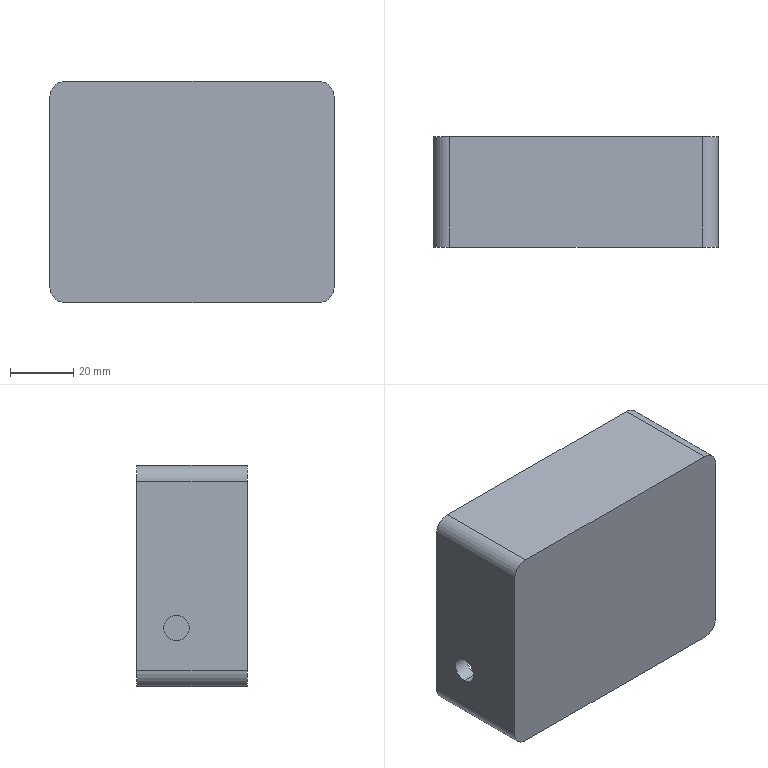Part | SolidWorks | features ICE 2, Extrusion 1, Fillet 1, HoleWzd 1 | 1 solid | 37 faces | box 90 x 35 x 70 mm | volume 61634 mm3 | cylinder 18 | plane 11 | cone 8 | commonest cylinder face diameters 2.5 x8 10 x8 8 x2
STEP:
#1=CARTESIAN_POINT('',(-40.,22.4,-20.5));
#2=VERTEX_POINT('',#1);
#3=CARTESIAN_POINT('',(-40.,22.4,-12.5));
#4=VERTEX_POINT('',#3);
#5=CARTESIAN_POINT('',(-40.,22.4,-16.5));
#6=DIRECTION('',(-1.,0.,0.));
#7=DIRECTION('',(0.,0.,1.));
#8=AXIS2_PLACEMENT_3D('',#5,#6,#7);
#9=CIRCLE('',#8,4.);
#10=EDGE_CURVE('',#2,#4,#9,.T.);
#11=ORIENTED_EDGE('',*,*,#10,.F.);
#12=CARTESIAN_POINT('',(-45.,22.4,-20.5));
#13=VERTEX_POINT('',#12);
#14=CARTESIAN_POINT('',(-35.,22.4,-20.5));
#15=DIRECTION('',(-1.,0.,0.));
#16=VECTOR('',#15,1000.);
#17=LINE('',#14,#16);
#18=EDGE_CURVE('',#2,#13,#17,.T.);
#19=ORIENTED_EDGE('',*,*,#18,.T.);
#20=CARTESIAN_POINT('',(-45.,22.4,-12.5));
#21=VERTEX_POINT('',#20);
#22=CARTESIAN_POINT('',(-45.,22.4,-16.5));
#23=DIRECTION('',(-1.,0.,0.));
#24=DIRECTION('',(0.,0.,1.));
#25=AXIS2_PLACEMENT_3D('',#22,#23,#24);
#26=CIRCLE('',#25,4.);
#27=EDGE_CURVE('',#13,#21,#26,.T.);
#28=ORIENTED_EDGE('',*,*,#27,.T.);
#29=CARTESIAN_POINT('',(-35.,22.4,-12.5));
#30=DIRECTION('',(-1.,0.,0.));
#31=VECTOR('',#30,1000.);
#32=LINE('',#29,#31);
#33=EDGE_CURVE('',#4,#21,#32,.T.);
#34=ORIENTED_EDGE('',*,*,#33,.F.);
#35=EDGE_LOOP('',(#11,#19,#28,#34));
#36=FACE_OUTER_BOUND('',#35,.T.);
#37=CARTESIAN_POINT('',(-35.,22.4,-16.5));
#38=DIRECTION('',(-1.,0.,0.));
#39=DIRECTION('',(0.,0.,1.));
#40=AXIS2_PLACEMENT_3D('',#37,#38,#39);
#41=CYLINDRICAL_SURFACE('',#40,4.);
#42=ADVANCED_FACE('',(#36),#41,.F.);
#43=CARTESIAN_POINT('',(-41.,26.5,-32.25));
#44=VERTEX_POINT('',#43);
#45=CARTESIAN_POINT('',(-41.,26.5,-29.75));
#46=VERTEX_POINT('',#45);
#47=CARTESIAN_POINT('',(-41.,26.5,-31.));
#48=DIRECTION('',(0.,1.,0.));
#49=DIRECTION('',(0.,0.,1.));
#50=AXIS2_PLACEMENT_3D('',#47,#48,#49);
#51=CIRCLE('',#50,1.25);
#52=EDGE_CURVE('',#44,#46,#51,.T.);
#53=ORIENTED_EDGE('',*,*,#52,.F.);
#54=CARTESIAN_POINT('',(-41.,35.,-32.25));
#55=VERTEX_POINT('',#54);
#56=CARTESIAN_POINT('',(-41.,35.,-32.25));
#57=DIRECTION('',(0.,1.,0.));
#58=VECTOR('',#57,1000.);
#59=LINE('',#56,#58);
#60=EDGE_CURVE('',#44,#55,#59,.T.);
#61=ORIENTED_EDGE('',*,*,#60,.T.);
#62=CARTESIAN_POINT('',(-41.,35.,-29.75));
#63=VERTEX_POINT('',#62);
#64=CARTESIAN_POINT('',(-41.,35.,-31.));
#65=DIRECTION('',(0.,1.,0.));
#66=DIRECTION('',(0.,0.,1.));
#67=AXIS2_PLACEMENT_3D('',#64,#65,#66);
#68=CIRCLE('',#67,1.25);
#69=EDGE_CURVE('',#55,#63,#68,.T.);
#70=ORIENTED_EDGE('',*,*,#69,.T.);
#71=CARTESIAN_POINT('',(-41.,35.,-29.75));
#72=DIRECTION('',(0.,1.,0.));
#73=VECTOR('',#72,1000.);
#74=LINE('',#71,#73);
#75=EDGE_CURVE('',#46,#63,#74,.T.);
#76=ORIENTED_EDGE('',*,*,#75,.F.);
#77=EDGE_LOOP('',(#53,#61,#70,#76));
#78=FACE_OUTER_BOUND('',#77,.T.);
#79=CARTESIAN_POINT('',(-41.,35.,-31.));
#80=DIRECTION('',(0.,1.,0.));
#81=DIRECTION('',(0.,0.,1.));
#82=AXIS2_PLACEMENT_3D('',#79,#80,#81);
#83=CYLINDRICAL_SURFACE('',#82,1.25);
#84=ADVANCED_FACE('',(#78),#83,.F.);
#85=CARTESIAN_POINT('',(-41.,25.749,-31.));
#86=VERTEX_POINT('',#85);
#87=CARTESIAN_POINT('',(-41.,26.5,-29.75));
#88=DIRECTION('',(0.,0.515,0.8572));
#89=VECTOR('',#88,1000.);
#90=LINE('',#87,#89);
#91=EDGE_CURVE('',#86,#46,#90,.T.);
#92=ORIENTED_EDGE('',*,*,#91,.F.);
#93=CARTESIAN_POINT('',(-41.,26.5,-32.25));
#94=DIRECTION('',(0.,0.515,-0.8572));
#95=VECTOR('',#94,1000.);
#96=LINE('',#93,#95);
#97=EDGE_CURVE('',#86,#44,#96,.T.);
#98=ORIENTED_EDGE('',*,*,#97,.T.);
#99=ORIENTED_EDGE('',*,*,#52,.T.);
#100=EDGE_LOOP('',(#92,#98,#99));
#101=FACE_OUTER_BOUND('',#100,.T.);
#102=CARTESIAN_POINT('',(-41.,26.5,-31.));
#103=DIRECTION('',(0.,1.,0.));
#104=DIRECTION('',(0.,0.,1.));
#105=AXIS2_PLACEMENT_3D('',#102,#103,#104);
#106=CONICAL_SURFACE('',#105,1.25,1.03);
#107=ADVANCED_FACE('',(#101),#106,.F.);
#108=CARTESIAN_POINT('',(41.,26.5,-32.25));
#109=VERTEX_POINT('',#108);
#110=CARTESIAN_POINT('',(41.,26.5,-29.75));
#111=VERTEX_POINT('',#110);
#112=CARTESIAN_POINT('',(41.,26.5,-31.));
#113=DIRECTION('',(0.,1.,0.));
#114=DIRECTION('',(0.,0.,1.));
#115=AXIS2_PLACEMENT_3D('',#112,#113,#114);
#116=CIRCLE('',#115,1.25);
#117=EDGE_CURVE('',#109,#111,#116,.T.);
#118=ORIENTED_EDGE('',*,*,#117,.F.);
#119=CARTESIAN_POINT('',(41.,35.,-32.25));
#120=VERTEX_POINT('',#119);
#121=CARTESIAN_POINT('',(41.,35.,-32.25));
#122=DIRECTION('',(0.,1.,0.));
#123=VECTOR('',#122,1000.);
#124=LINE('',#121,#123);
#125=EDGE_CURVE('',#109,#120,#124,.T.);
#126=ORIENTED_EDGE('',*,*,#125,.T.);
#127=CARTESIAN_POINT('',(41.,35.,-29.75));
#128=VERTEX_POINT('',#127);
#129=CARTESIAN_POINT('',(41.,35.,-31.));
#130=DIRECTION('',(0.,1.,0.));
#131=DIRECTION('',(0.,0.,1.));
#132=AXIS2_PLACEMENT_3D('',#129,#130,#131);
#133=CIRCLE('',#132,1.25);
#134=EDGE_CURVE('',#120,#128,#133,.T.);
#135=ORIENTED_EDGE('',*,*,#134,.T.);
#136=CARTESIAN_POINT('',(41.,35.,-29.75));
#137=DIRECTION('',(0.,1.,0.));
#138=VECTOR('',#137,1000.);
#139=LINE('',#136,#138);
#140=EDGE_CURVE('',#111,#128,#139,.T.);
#141=ORIENTED_EDGE('',*,*,#140,.F.);
#142=EDGE_LOOP('',(#118,#126,#135,#141));
#143=FACE_OUTER_BOUND('',#142,.T.);
#144=CARTESIAN_POINT('',(41.,35.,-31.));
#145=DIRECTION('',(0.,1.,0.));
#146=DIRECTION('',(0.,0.,1.));
#147=AXIS2_PLACEMENT_3D('',#144,#145,#146);
#148=CYLINDRICAL_SURFACE('',#147,1.25);
#149=ADVANCED_FACE('',(#143),#148,.F.);
#150=CARTESIAN_POINT('',(41.,25.749,-31.));
#151=VERTEX_POINT('',#150);
#152=CARTESIAN_POINT('',(41.,26.5,-29.75));
#153=DIRECTION('',(0.,0.515,0.8572));
#154=VECTOR('',#153,1000.);
#155=LINE('',#152,#154);
#156=EDGE_CURVE('',#151,#111,#155,.T.);
#157=ORIENTED_EDGE('',*,*,#156,.F.);
#158=CARTESIAN_POINT('',(41.,26.5,-32.25));
#159=DIRECTION('',(0.,0.515,-0.8572));
#160=VECTOR('',#159,1000.);
#161=LINE('',#158,#160);
#162=EDGE_CURVE('',#151,#109,#161,.T.);
#163=ORIENTED_EDGE('',*,*,#162,.T.);
#164=ORIENTED_EDGE('',*,*,#117,.T.);
#165=EDGE_LOOP('',(#157,#163,#164));
#166=FACE_OUTER_BOUND('',#165,.T.);
#167=CARTESIAN_POINT('',(41.,26.5,-31.));
#168=DIRECTION('',(0.,1.,0.));
#169=DIRECTION('',(0.,0.,1.));
#170=AXIS2_PLACEMENT_3D('',#167,#168,#169);
#171=CONICAL_SURFACE('',#170,1.25,1.03);
#172=ADVANCED_FACE('',(#166),#171,.F.);
#173=CARTESIAN_POINT('',(41.,26.5,29.75));
#174=VERTEX_POINT('',#173);
#175=CARTESIAN_POINT('',(41.,26.5,32.25));
#176=VERTEX_POINT('',#175);
#177=CARTESIAN_POINT('',(41.,26.5,31.));
#178=DIRECTION('',(0.,1.,0.));
#179=DIRECTION('',(0.,0.,1.));
#180=AXIS2_PLACEMENT_3D('',#177,#178,#179);
#181=CIRCLE('',#180,1.25);
#182=EDGE_CURVE('',#174,#176,#181,.T.);
#183=ORIENTED_EDGE('',*,*,#182,.F.);
#184=CARTESIAN_POINT('',(41.,35.,29.75));
#185=VERTEX_POINT('',#184);
#186=CARTESIAN_POINT('',(41.,35.,29.75));
#187=DIRECTION('',(0.,1.,0.));
#188=VECTOR('',#187,1000.);
#189=LINE('',#186,#188);
#190=EDGE_CURVE('',#174,#185,#189,.T.);
#191=ORIENTED_EDGE('',*,*,#190,.T.);
#192=CARTESIAN_POINT('',(41.,35.,32.25));
#193=VERTEX_POINT('',#192);
#194=CARTESIAN_POINT('',(41.,35.,31.));
#195=DIRECTION('',(0.,1.,0.));
#196=DIRECTION('',(0.,0.,1.));
#197=AXIS2_PLACEMENT_3D('',#194,#195,#196);
#198=CIRCLE('',#197,1.25);
#199=EDGE_CURVE('',#185,#193,#198,.T.);
#200=ORIENTED_EDGE('',*,*,#199,.T.);
#201=CARTESIAN_POINT('',(41.,35.,32.25));
#202=DIRECTION('',(0.,1.,0.));
#203=VECTOR('',#202,1000.);
#204=LINE('',#201,#203);
#205=EDGE_CURVE('',#176,#193,#204,.T.);
#206=ORIENTED_EDGE('',*,*,#205,.F.);
#207=EDGE_LOOP('',(#183,#191,#200,#206));
#208=FACE_OUTER_BOUND('',#207,.T.);
#209=CARTESIAN_POINT('',(41.,35.,31.));
#210=DIRECTION('',(0.,1.,0.));
#211=DIRECTION('',(0.,0.,1.));
#212=AXIS2_PLACEMENT_3D('',#209,#210,#211);
#213=CYLINDRICAL_SURFACE('',#212,1.25);
#214=ADVANCED_FACE('',(#208),#213,.F.);
#215=CARTESIAN_POINT('',(41.,25.749,31.));
#216=VERTEX_POINT('',#215);
#217=CARTESIAN_POINT('',(41.,26.5,32.25));
#218=DIRECTION('',(0.,0.515,0.8572));
#219=VECTOR('',#218,1000.);
#220=LINE('',#217,#219);
#221=EDGE_CURVE('',#216,#176,#220,.T.);
#222=ORIENTED_EDGE('',*,*,#221,.F.);
#223=CARTESIAN_POINT('',(41.,26.5,29.75));
#224=DIRECTION('',(0.,0.515,-0.8572));
#225=VECTOR('',#224,1000.);
#226=LINE('',#223,#225);
#227=EDGE_CURVE('',#216,#174,#226,.T.);
#228=ORIENTED_EDGE('',*,*,#227,.T.);
#229=ORIENTED_EDGE('',*,*,#182,.T.);
#230=EDGE_LOOP('',(#222,#228,#229));
#231=FACE_OUTER_BOUND('',#230,.T.);
#232=CARTESIAN_POINT('',(41.,26.5,31.));
#233=DIRECTION('',(0.,1.,0.));
#234=DIRECTION('',(0.,0.,1.));
#235=AXIS2_PLACEMENT_3D('',#232,#233,#234);
#236=CONICAL_SURFACE('',#235,1.25,1.03);
#237=ADVANCED_FACE('',(#231),#236,.F.);
#238=CARTESIAN_POINT('',(-41.,26.5,29.75));
#239=VERTEX_POINT('',#238);
#240=CARTESIAN_POINT('',(-41.,26.5,32.25));
#241=VERTEX_POINT('',#240);
#242=CARTESIAN_POINT('',(-41.,26.5,31.));
#243=DIRECTION('',(0.,1.,0.));
#244=DIRECTION('',(0.,0.,1.));
#245=AXIS2_PLACEMENT_3D('',#242,#243,#244);
#246=CIRCLE('',#245,1.25);
#247=EDGE_CURVE('',#239,#241,#246,.T.);
#248=ORIENTED_EDGE('',*,*,#247,.F.);
#249=CARTESIAN_POINT('',(-41.,35.,29.75));
#250=VERTEX_POINT('',#249);
#251=CARTESIAN_POINT('',(-41.,35.,29.75));
#252=DIRECTION('',(0.,1.,0.));
#253=VECTOR('',#252,1000.);
#254=LINE('',#251,#253);
#255=EDGE_CURVE('',#239,#250,#254,.T.);
#256=ORIENTED_EDGE('',*,*,#255,.T.);
#257=CARTESIAN_POINT('',(-41.,35.,32.25));
#258=VERTEX_POINT('',#257);
#259=CARTESIAN_POINT('',(-41.,35.,31.));
#260=DIRECTION('',(0.,1.,0.));
#261=DIRECTION('',(0.,0.,1.));
#262=AXIS2_PLACEMENT_3D('',#259,#260,#261);
#263=CIRCLE('',#262,1.25);
#264=EDGE_CURVE('',#250,#258,#263,.T.);
#265=ORIENTED_EDGE('',*,*,#264,.T.);
#266=CARTESIAN_POINT('',(-41.,35.,32.25));
#267=DIRECTION('',(0.,1.,0.));
#268=VECTOR('',#267,1000.);
#269=LINE('',#266,#268);
#270=EDGE_CURVE('',#241,#258,#269,.T.);
#271=ORIENTED_EDGE('',*,*,#270,.F.);
#272=EDGE_LOOP('',(#248,#256,#265,#271));
#273=FACE_OUTER_BOUND('',#272,.T.);
#274=CARTESIAN_POINT('',(-41.,35.,31.));
#275=DIRECTION('',(0.,1.,0.));
#276=DIRECTION('',(0.,0.,1.));
#277=AXIS2_PLACEMENT_3D('',#274,#275,#276);
#278=CYLINDRICAL_SURFACE('',#277,1.25);
#279=ADVANCED_FACE('',(#273),#278,.F.);
#280=CARTESIAN_POINT('',(-41.,25.749,31.));
#281=VERTEX_POINT('',#280);
#282=CARTESIAN_POINT('',(-41.,26.5,32.25));
#283=DIRECTION('',(0.,0.515,0.8572));
#284=VECTOR('',#283,1000.);
#285=LINE('',#282,#284);
#286=EDGE_CURVE('',#281,#241,#285,.T.);
#287=ORIENTED_EDGE('',*,*,#286,.F.);
#288=CARTESIAN_POINT('',(-41.,26.5,29.75));
#289=DIRECTION('',(0.,0.515,-0.8572));
#290=VECTOR('',#289,1000.);
#291=LINE('',#288,#290);
#292=EDGE_CURVE('',#281,#239,#291,.T.);
#293=ORIENTED_EDGE('',*,*,#292,.T.);
#294=ORIENTED_EDGE('',*,*,#247,.T.);
#295=EDGE_LOOP('',(#287,#293,#294));
#296=FACE_OUTER_BOUND('',#295,.T.);
#297=CARTESIAN_POINT('',(-41.,26.5,31.));
#298=DIRECTION('',(0.,1.,0.));
#299=DIRECTION('',(0.,0.,1.));
#300=AXIS2_PLACEMENT_3D('',#297,#298,#299);
#301=CONICAL_SURFACE('',#300,1.25,1.03);
#302=ADVANCED_FACE('',(#296),#301,.F.);
#303=CARTESIAN_POINT('',(-41.,35.,-31.));
#304=DIRECTION('',(0.,1.,0.));
#305=DIRECTION('',(0.,0.,1.));
#306=AXIS2_PLACEMENT_3D('',#303,#304,#305);
#307=CIRCLE('',#306,1.25);
#308=EDGE_CURVE('',#63,#55,#307,.T.);
#309=ORIENTED_EDGE('',*,*,#308,.F.);
#310=ORIENTED_EDGE('',*,*,#69,.F.);
#311=EDGE_LOOP('',(#309,#310));
#312=FACE_BOUND('',#311,.T.);
#313=CARTESIAN_POINT('',(41.,35.,-31.));
#314=DIRECTION('',(0.,1.,0.));
#315=DIRECTION('',(0.,0.,1.));
#316=AXIS2_PLACEMENT_3D('',#313,#314,#315);
#317=CIRCLE('',#316,1.25);
#318=EDGE_CURVE('',#128,#120,#317,.T.);
#319=ORIENTED_EDGE('',*,*,#318,.F.);
#320=ORIENTED_EDGE('',*,*,#134,.F.);
#321=EDGE_LOOP('',(#319,#320));
#322=FACE_BOUND('',#321,.T.);
#323=CARTESIAN_POINT('',(-41.,35.,31.));
#324=DIRECTION('',(0.,1.,0.));
#325=DIRECTION('',(0.,0.,1.));
#326=AXIS2_PLACEMENT_3D('',#323,#324,#325);
#327=CIRCLE('',#326,1.25);
#328=EDGE_CURVE('',#258,#250,#327,.T.);
#329=ORIENTED_EDGE('',*,*,#328,.F.);
#330=ORIENTED_EDGE('',*,*,#264,.F.);
#331=EDGE_LOOP('',(#329,#330));
#332=FACE_BOUND('',#331,.T.);
#333=CARTESIAN_POINT('',(35.,35.,-30.));
#334=VERTEX_POINT('',#333);
#335=CARTESIAN_POINT('',(-35.,35.,-30.));
#336=VERTEX_POINT('',#335);
#337=CARTESIAN_POINT('',(-40.,35.,-30.));
#338=DIRECTION('',(-1.,0.,0.));
#339=VECTOR('',#338,1000.);
#340=LINE('',#337,#339);
#341=EDGE_CURVE('',#334,#336,#340,.T.);
#342=ORIENTED_EDGE('',*,*,#341,.F.);
#343=CARTESIAN_POINT('',(40.,35.,-25.));
#344=VERTEX_POINT('',#343);
#345=CARTESIAN_POINT('',(35.,35.,-25.));
#346=DIRECTION('',(0.,-1.,0.));
#347=DIRECTION('',(0.,0.,-1.));
#348=AXIS2_PLACEMENT_3D('',#345,#346,#347);
#349=CIRCLE('',#348,5.);
#350=EDGE_CURVE('',#334,#344,#349,.T.);
#351=ORIENTED_EDGE('',*,*,#350,.T.);
#352=CARTESIAN_POINT('',(40.,35.,25.));
#353=VERTEX_POINT('',#352);
#354=CARTESIAN_POINT('',(40.,35.,30.));
#355=DIRECTION('',(0.,0.,-1.));
#356=VECTOR('',#355,1000.);
#357=LINE('',#354,#356);
#358=EDGE_CURVE('',#353,#344,#357,.T.);
#359=ORIENTED_EDGE('',*,*,#358,.F.);
#360=CARTESIAN_POINT('',(35.,35.,30.));
#361=VERTEX_POINT('',#360);
#362=CARTESIAN_POINT('',(35.,35.,25.));
#363=DIRECTION('',(0.,-1.,0.));
#364=DIRECTION('',(0.,0.,-1.));
#365=AXIS2_PLACEMENT_3D('',#362,#363,#364);
#366=CIRCLE('',#365,5.);
#367=EDGE_CURVE('',#353,#361,#366,.T.);
#368=ORIENTED_EDGE('',*,*,#367,.T.);
#369=CARTESIAN_POINT('',(-35.,35.,30.));
#370=VERTEX_POINT('',#369);
#371=CARTESIAN_POINT('',(-40.,35.,30.));
#372=DIRECTION('',(1.,0.,0.));
#373=VECTOR('',#372,1000.);
#374=LINE('',#371,#373);
#375=EDGE_CURVE('',#370,#361,#374,.T.);
#376=ORIENTED_EDGE('',*,*,#375,.F.);
#377=CARTESIAN_POINT('',(-40.,35.,25.));
#378=VERTEX_POINT('',#377);
#379=CARTESIAN_POINT('',(-35.,35.,25.));
#380=DIRECTION('',(0.,-1.,0.));
#381=DIRECTION('',(0.,0.,-1.));
#382=AXIS2_PLACEMENT_3D('',#379,#380,#381);
#383=CIRCLE('',#382,5.);
#384=EDGE_CURVE('',#370,#378,#383,.T.);
#385=ORIENTED_EDGE('',*,*,#384,.T.);
#386=CARTESIAN_POINT('',(-40.,35.,-25.));
#387=VERTEX_POINT('',#386);
#388=CARTESIAN_POINT('',(-40.,35.,30.));
#389=DIRECTION('',(0.,0.,1.));
#390=VECTOR('',#389,1000.);
#391=LINE('',#388,#390);
#392=EDGE_CURVE('',#387,#378,#391,.T.);
#393=ORIENTED_EDGE('',*,*,#392,.F.);
#394=CARTESIAN_POINT('',(-35.,35.,-25.));
#395=DIRECTION('',(0.,-1.,0.));
#396=DIRECTION('',(0.,0.,-1.));
#397=AXIS2_PLACEMENT_3D('',#394,#395,#396);
#398=CIRCLE('',#397,5.);
#399=EDGE_CURVE('',#387,#336,#398,.T.);
#400=ORIENTED_EDGE('',*,*,#399,.T.);
#401=EDGE_LOOP('',(#342,#351,#359,#368,#376,#385,#393,#400));
#402=FACE_BOUND('',#401,.T.);
#403=CARTESIAN_POINT('',(45.,35.,30.));
#404=VERTEX_POINT('',#403);
#405=CARTESIAN_POINT('',(45.,35.,-30.));
#406=VERTEX_POINT('',#405);
#407=CARTESIAN_POINT('',(45.,35.,35.));
#408=DIRECTION('',(0.,0.,-1.));
#409=VECTOR('',#408,1000.);
#410=LINE('',#407,#409);
#411=EDGE_CURVE('',#404,#406,#410,.T.);
#412=ORIENTED_EDGE('',*,*,#411,.T.);
#413=CARTESIAN_POINT('',(40.,35.,-35.));
#414=VERTEX_POINT('',#413);
#415=CARTESIAN_POINT('',(40.,35.,-30.));
#416=DIRECTION('',(0.,1.,0.));
#417=DIRECTION('',(0.,0.,-1.));
#418=AXIS2_PLACEMENT_3D('',#415,#416,#417);
#419=CIRCLE('',#418,5.);
#420=EDGE_CURVE('',#406,#414,#419,.T.);
#421=ORIENTED_EDGE('',*,*,#420,.T.);
#422=CARTESIAN_POINT('',(-40.,35.,-35.));
#423=VERTEX_POINT('',#422);
#424=CARTESIAN_POINT('',(-45.,35.,-35.));
#425=DIRECTION('',(-1.,0.,0.));
#426=VECTOR('',#425,1000.);
#427=LINE('',#424,#426);
#428=EDGE_CURVE('',#414,#423,#427,.T.);
#429=ORIENTED_EDGE('',*,*,#428,.T.);
#430=CARTESIAN_POINT('',(-45.,35.,-30.));
#431=VERTEX_POINT('',#430);
#432=CARTESIAN_POINT('',(-40.,35.,-30.));
#433=DIRECTION('',(0.,1.,0.));
#434=DIRECTION('',(0.,0.,-1.));
#435=AXIS2_PLACEMENT_3D('',#432,#433,#434);
#436=CIRCLE('',#435,5.);
#437=EDGE_CURVE('',#423,#431,#436,.T.);
#438=ORIENTED_EDGE('',*,*,#437,.T.);
#439=CARTESIAN_POINT('',(-45.,35.,30.));
#440=VERTEX_POINT('',#439);
#441=CARTESIAN_POINT('',(-45.,35.,35.));
#442=DIRECTION('',(0.,0.,1.));
#443=VECTOR('',#442,1000.);
#444=LINE('',#441,#443);
#445=EDGE_CURVE('',#431,#440,#444,.T.);
#446=ORIENTED_EDGE('',*,*,#445,.T.);
#447=CARTESIAN_POINT('',(-40.,35.,35.));
#448=VERTEX_POINT('',#447);
#449=CARTESIAN_POINT('',(-40.,35.,30.));
#450=DIRECTION('',(0.,1.,0.));
#451=DIRECTION('',(0.,0.,-1.));
#452=AXIS2_PLACEMENT_3D('',#449,#450,#451);
#453=CIRCLE('',#452,5.);
#454=EDGE_CURVE('',#440,#448,#453,.T.);
#455=ORIENTED_EDGE('',*,*,#454,.T.);
#456=CARTESIAN_POINT('',(40.,35.,35.));
#457=VERTEX_POINT('',#456);
#458=CARTESIAN_POINT('',(-45.,35.,35.));
#459=DIRECTION('',(1.,0.,0.));
#460=VECTOR('',#459,1000.);
#461=LINE('',#458,#460);
#462=EDGE_CURVE('',#448,#457,#461,.T.);
#463=ORIENTED_EDGE('',*,*,#462,.T.);
#464=CARTESIAN_POINT('',(40.,35.,30.));
#465=DIRECTION('',(0.,1.,0.));
#466=DIRECTION('',(0.,0.,-1.));
#467=AXIS2_PLACEMENT_3D('',#464,#465,#466);
#468=CIRCLE('',#467,5.);
#469=EDGE_CURVE('',#457,#404,#468,.T.);
#470=ORIENTED_EDGE('',*,*,#469,.T.);
#471=EDGE_LOOP('',(#412,#421,#429,#438,#446,#455,#463,#470));
#472=FACE_OUTER_BOUND('',#471,.T.);
#473=CARTESIAN_POINT('',(41.,35.,31.));
#474=DIRECTION('',(0.,1.,0.));
#475=DIRECTION('',(0.,0.,1.));
#476=AXIS2_PLACEMENT_3D('',#473,#474,#475);
#477=CIRCLE('',#476,1.25);
#478=EDGE_CURVE('',#193,#185,#477,.T.);
#479=ORIENTED_EDGE('',*,*,#478,.F.);
#480=ORIENTED_EDGE('',*,*,#199,.F.);
#481=EDGE_LOOP('',(#479,#480));
#482=FACE_BOUND('',#481,.T.);
#483=CARTESIAN_POINT('',(0.,35.,0.));
#484=DIRECTION('',(0.,-1.,0.));
#485=DIRECTION('',(0.,0.,-1.));
#486=AXIS2_PLACEMENT_3D('',#483,#484,#485);
#487=PLANE('',#486);
#488=ADVANCED_FACE('',(#312,#322,#332,#402,#472,#482),#487,.F.);
#489=CARTESIAN_POINT('',(45.,0.,30.));
#490=VERTEX_POINT('',#489);
#491=CARTESIAN_POINT('',(45.,0.,-30.));
#492=VERTEX_POINT('',#491);
#493=CARTESIAN_POINT('',(45.,0.,35.));
#494=DIRECTION('',(0.,0.,-1.));
#495=VECTOR('',#494,1000.);
#496=LINE('',#493,#495);
#497=EDGE_CURVE('',#490,#492,#496,.T.);
#498=ORIENTED_EDGE('',*,*,#497,.T.);
#499=CARTESIAN_POINT('',(45.,35.,-30.));
#500=DIRECTION('',(0.,1.,0.));
#501=VECTOR('',#500,1000.);
#502=LINE('',#499,#501);
#503=EDGE_CURVE('',#492,#406,#502,.T.);
#504=ORIENTED_EDGE('',*,*,#503,.T.);
#505=ORIENTED_EDGE('',*,*,#411,.F.);
#506=CARTESIAN_POINT('',(45.,35.,30.));
#507=DIRECTION('',(0.,-1.,0.));
#508=VECTOR('',#507,1000.);
#509=LINE('',#506,#508);
#510=EDGE_CURVE('',#404,#490,#509,.T.);
#511=ORIENTED_EDGE('',*,*,#510,.T.);
#512=EDGE_LOOP('',(#498,#504,#505,#511));
#513=FACE_OUTER_BOUND('',#512,.T.);
#514=CARTESIAN_POINT('',(45.,35.,35.));
#515=DIRECTION('',(-1.,0.,0.));
#516=DIRECTION('',(0.,0.,1.));
#517=AXIS2_PLACEMENT_3D('',#514,#515,#516);
#518=PLANE('',#517);
#519=ADVANCED_FACE('',(#513),#518,.F.);
#520=ORIENTED_EDGE('',*,*,#428,.F.);
#521=CARTESIAN_POINT('',(40.,0.,-35.));
#522=VERTEX_POINT('',#521);
#523=CARTESIAN_POINT('',(40.,35.,-35.));
#524=DIRECTION('',(0.,-1.,0.));
#525=VECTOR('',#524,1000.);
#526=LINE('',#523,#525);
#527=EDGE_CURVE('',#414,#522,#526,.T.);
#528=ORIENTED_EDGE('',*,*,#527,.T.);
#529=CARTESIAN_POINT('',(-40.,0.,-35.));
#530=VERTEX_POINT('',#529);
#531=CARTESIAN_POINT('',(-45.,0.,-35.));
#532=DIRECTION('',(-1.,0.,0.));
#533=VECTOR('',#532,1000.);
#534=LINE('',#531,#533);
#535=EDGE_CURVE('',#522,#530,#534,.T.);
#536=ORIENTED_EDGE('',*,*,#535,.T.);
#537=CARTESIAN_POINT('',(-40.,35.,-35.));
#538=DIRECTION('',(0.,1.,0.));
#539=VECTOR('',#538,1000.);
#540=LINE('',#537,#539);
#541=EDGE_CURVE('',#530,#423,#540,.T.);
#542=ORIENTED_EDGE('',*,*,#541,.T.);
#543=EDGE_LOOP('',(#520,#528,#536,#542));
#544=FACE_OUTER_BOUND('',#543,.T.);
#545=CARTESIAN_POINT('',(-45.,35.,-35.));
#546=DIRECTION('',(0.,0.,1.));
#547=DIRECTION('',(1.,0.,0.));
#548=AXIS2_PLACEMENT_3D('',#545,#546,#547);
#549=PLANE('',#548);
#550=ADVANCED_FACE('',(#544),#549,.F.);
#551=CARTESIAN_POINT('',(-45.,22.4,-16.5));
#552=DIRECTION('',(-1.,0.,0.));
#553=DIRECTION('',(0.,0.,1.));
#554=AXIS2_PLACEMENT_3D('',#551,#552,#553);
#555=CIRCLE('',#554,4.);
#556=EDGE_CURVE('',#21,#13,#555,.T.);
#557=ORIENTED_EDGE('',*,*,#556,.F.);
#558=ORIENTED_EDGE('',*,*,#27,.F.);
#559=EDGE_LOOP('',(#557,#558));
#560=FACE_BOUND('',#559,.T.);
#561=CARTESIAN_POINT('',(-45.,0.,-30.));
#562=VERTEX_POINT('',#561);
#563=CARTESIAN_POINT('',(-45.,0.,30.));
#564=VERTEX_POINT('',#563);
#565=CARTESIAN_POINT('',(-45.,0.,35.));
#566=DIRECTION('',(0.,0.,1.));
#567=VECTOR('',#566,1000.);
#568=LINE('',#565,#567);
#569=EDGE_CURVE('',#562,#564,#568,.T.);
#570=ORIENTED_EDGE('',*,*,#569,.T.);
#571=CARTESIAN_POINT('',(-45.,35.,30.));
#572=DIRECTION('',(0.,1.,0.));
#573=VECTOR('',#572,1000.);
#574=LINE('',#571,#573);
#575=EDGE_CURVE('',#564,#440,#574,.T.);
#576=ORIENTED_EDGE('',*,*,#575,.T.);
#577=ORIENTED_EDGE('',*,*,#445,.F.);
#578=CARTESIAN_POINT('',(-45.,35.,-30.));
#579=DIRECTION('',(0.,-1.,0.));
#580=VECTOR('',#579,1000.);
#581=LINE('',#578,#580);
#582=EDGE_CURVE('',#431,#562,#581,.T.);
#583=ORIENTED_EDGE('',*,*,#582,.T.);
#584=EDGE_LOOP('',(#570,#576,#577,#583));
#585=FACE_OUTER_BOUND('',#584,.T.);
#586=CARTESIAN_POINT('',(-45.,35.,35.));
#587=DIRECTION('',(1.,0.,0.));
#588=DIRECTION('',(0.,0.,-1.));
#589=AXIS2_PLACEMENT_3D('',#586,#587,#588);
#590=PLANE('',#589);
#591=ADVANCED_FACE('',(#560,#585),#590,.F.);
#592=CARTESIAN_POINT('',(-40.,0.,35.));
#593=VERTEX_POINT('',#592);
#594=CARTESIAN_POINT('',(40.,0.,35.));
#595=VERTEX_POINT('',#594);
#596=CARTESIAN_POINT('',(-45.,0.,35.));
#597=DIRECTION('',(1.,0.,0.));
#598=VECTOR('',#597,1000.);
#599=LINE('',#596,#598);
#600=EDGE_CURVE('',#593,#595,#599,.T.);
#601=ORIENTED_EDGE('',*,*,#600,.T.);
#602=CARTESIAN_POINT('',(40.,35.,35.));
#603=DIRECTION('',(0.,1.,0.));
#604=VECTOR('',#603,1000.);
#605=LINE('',#602,#604);
#606=EDGE_CURVE('',#595,#457,#605,.T.);
#607=ORIENTED_EDGE('',*,*,#606,.T.);
#608=ORIENTED_EDGE('',*,*,#462,.F.);
#609=CARTESIAN_POINT('',(-40.,35.,35.));
#610=DIRECTION('',(0.,-1.,0.));
#611=VECTOR('',#610,1000.);
#612=LINE('',#609,#611);
#613=EDGE_CURVE('',#448,#593,#612,.T.);
#614=ORIENTED_EDGE('',*,*,#613,.T.);
#615=EDGE_LOOP('',(#601,#607,#608,#614));
#616=FACE_OUTER_BOUND('',#615,.T.);
#617=CARTESIAN_POINT('',(-45.,35.,35.));
#618=DIRECTION('',(0.,0.,-1.));
#619=DIRECTION('',(-1.,0.,0.));
#620=AXIS2_PLACEMENT_3D('',#617,#618,#619);
#621=PLANE('',#620);
#622=ADVANCED_FACE('',(#616),#621,.F.);
#623=ORIENTED_EDGE('',*,*,#535,.F.);
#624=CARTESIAN_POINT('',(40.,0.,-30.));
#625=DIRECTION('',(0.,-1.,0.));
#626=DIRECTION('',(0.,0.,-1.));
#627=AXIS2_PLACEMENT_3D('',#624,#625,#626);
#628=CIRCLE('',#627,5.);
#629=EDGE_CURVE('',#522,#492,#628,.T.);
#630=ORIENTED_EDGE('',*,*,#629,.T.);
#631=ORIENTED_EDGE('',*,*,#497,.F.);
#632=CARTESIAN_POINT('',(40.,0.,30.));
#633=DIRECTION('',(0.,-1.,0.));
#634=DIRECTION('',(0.,0.,-1.));
#635=AXIS2_PLACEMENT_3D('',#632,#633,#634);
#636=CIRCLE('',#635,5.);
#637=EDGE_CURVE('',#490,#595,#636,.T.);
#638=ORIENTED_EDGE('',*,*,#637,.T.);
#639=ORIENTED_EDGE('',*,*,#600,.F.);
#640=CARTESIAN_POINT('',(-40.,0.,30.));
#641=DIRECTION('',(0.,-1.,0.));
#642=DIRECTION('',(0.,0.,-1.));
#643=AXIS2_PLACEMENT_3D('',#640,#641,#642);
#644=CIRCLE('',#643,5.);
#645=EDGE_CURVE('',#593,#564,#644,.T.);
#646=ORIENTED_EDGE('',*,*,#645,.T.);
#647=ORIENTED_EDGE('',*,*,#569,.F.);
#648=CARTESIAN_POINT('',(-40.,0.,-30.));
#649=DIRECTION('',(0.,-1.,0.));
#650=DIRECTION('',(0.,0.,-1.));
#651=AXIS2_PLACEMENT_3D('',#648,#649,#650);
#652=CIRCLE('',#651,5.);
#653=EDGE_CURVE('',#562,#530,#652,.T.);
#654=ORIENTED_EDGE('',*,*,#653,.T.);
#655=EDGE_LOOP('',(#623,#630,#631,#638,#639,#646,#647,#654));
#656=FACE_OUTER_BOUND('',#655,.T.);
#657=CARTESIAN_POINT('',(0.,0.,0.));
#658=DIRECTION('',(0.,-1.,0.));
#659=DIRECTION('',(0.,0.,-1.));
#660=AXIS2_PLACEMENT_3D('',#657,#658,#659);
#661=PLANE('',#660);
#662=ADVANCED_FACE('',(#656),#661,.T.);
#663=CARTESIAN_POINT('',(40.,2.,25.));
#664=VERTEX_POINT('',#663);
#665=CARTESIAN_POINT('',(40.,2.,-25.));
#666=VERTEX_POINT('',#665);
#667=CARTESIAN_POINT('',(40.,2.,30.));
#668=DIRECTION('',(0.,0.,-1.));
#669=VECTOR('',#668,1000.);
#670=LINE('',#667,#669);
#671=EDGE_CURVE('',#664,#666,#670,.T.);
#672=ORIENTED_EDGE('',*,*,#671,.F.);
#673=CARTESIAN_POINT('',(40.,35.,25.));
#674=DIRECTION('',(0.,1.,0.));
#675=VECTOR('',#674,1000.);
#676=LINE('',#673,#675);
#677=EDGE_CURVE('',#664,#353,#676,.T.);
#678=ORIENTED_EDGE('',*,*,#677,.T.);
#679=ORIENTED_EDGE('',*,*,#358,.T.);
#680=CARTESIAN_POINT('',(40.,2.,-25.));
#681=DIRECTION('',(0.,-1.,0.));
#682=VECTOR('',#681,1000.);
#683=LINE('',#680,#682);
#684=EDGE_CURVE('',#344,#666,#683,.T.);
#685=ORIENTED_EDGE('',*,*,#684,.T.);
#686=EDGE_LOOP('',(#672,#678,#679,#685));
#687=FACE_OUTER_BOUND('',#686,.T.);
#688=CARTESIAN_POINT('',(40.,2.,30.));
#689=DIRECTION('',(1.,0.,0.));
#690=DIRECTION('',(0.,0.,-1.));
#691=AXIS2_PLACEMENT_3D('',#688,#689,#690);
#692=PLANE('',#691);
#693=ADVANCED_FACE('',(#687),#692,.F.);
#694=CARTESIAN_POINT('',(-35.,2.,30.));
#695=VERTEX_POINT('',#694);
#696=CARTESIAN_POINT('',(35.,2.,30.));
#697=VERTEX_POINT('',#696);
#698=CARTESIAN_POINT('',(-40.,2.,30.));
#699=DIRECTION('',(1.,0.,0.));
#700=VECTOR('',#699,1000.);
#701=LINE('',#698,#700);
#702=EDGE_CURVE('',#695,#697,#701,.T.);
#703=ORIENTED_EDGE('',*,*,#702,.F.);
#704=CARTESIAN_POINT('',(-35.,35.,30.));
#705=DIRECTION('',(0.,1.,0.));
#706=VECTOR('',#705,1000.);
#707=LINE('',#704,#706);
#708=EDGE_CURVE('',#695,#370,#707,.T.);
#709=ORIENTED_EDGE('',*,*,#708,.T.);
#710=ORIENTED_EDGE('',*,*,#375,.T.);
#711=CARTESIAN_POINT('',(35.,2.,30.));
#712=DIRECTION('',(0.,-1.,0.));
#713=VECTOR('',#712,1000.);
#714=LINE('',#711,#713);
#715=EDGE_CURVE('',#361,#697,#714,.T.);
#716=ORIENTED_EDGE('',*,*,#715,.T.);
#717=EDGE_LOOP('',(#703,#709,#710,#716));
#718=FACE_OUTER_BOUND('',#717,.T.);
#719=CARTESIAN_POINT('',(-40.,2.,30.));
#720=DIRECTION('',(0.,0.,1.));
#721=DIRECTION('',(1.,0.,0.));
#722=AXIS2_PLACEMENT_3D('',#719,#720,#721);
#723=PLANE('',#722);
#724=ADVANCED_FACE('',(#718),#723,.F.);
#725=CARTESIAN_POINT('',(-40.,22.4,-16.5));
#726=DIRECTION('',(-1.,0.,0.));
#727=DIRECTION('',(0.,0.,1.));
#728=AXIS2_PLACEMENT_3D('',#725,#726,#727);
#729=CIRCLE('',#728,4.);
#730=EDGE_CURVE('',#4,#2,#729,.T.);
#731=ORIENTED_EDGE('',*,*,#730,.T.);
#732=ORIENTED_EDGE('',*,*,#10,.T.);
#733=EDGE_LOOP('',(#731,#732));
#734=FACE_BOUND('',#733,.T.);
#735=ORIENTED_EDGE('',*,*,#392,.T.);
#736=CARTESIAN_POINT('',(-40.,2.,25.));
#737=VERTEX_POINT('',#736);
#738=CARTESIAN_POINT('',(-40.,2.,25.));
#739=DIRECTION('',(0.,-1.,0.));
#740=VECTOR('',#739,1000.);
#741=LINE('',#738,#740);
#742=EDGE_CURVE('',#378,#737,#741,.T.);
#743=ORIENTED_EDGE('',*,*,#742,.T.);
#744=CARTESIAN_POINT('',(-40.,2.,-25.));
#745=VERTEX_POINT('',#744);
#746=CARTESIAN_POINT('',(-40.,2.,30.));
#747=DIRECTION('',(0.,0.,1.));
#748=VECTOR('',#747,1000.);
#749=LINE('',#746,#748);
#750=EDGE_CURVE('',#745,#737,#749,.T.);
#751=ORIENTED_EDGE('',*,*,#750,.F.);
#752=CARTESIAN_POINT('',(-40.,35.,-25.));
#753=DIRECTION('',(0.,1.,0.));
#754=VECTOR('',#753,1000.);
#755=LINE('',#752,#754);
#756=EDGE_CURVE('',#745,#387,#755,.T.);
#757=ORIENTED_EDGE('',*,*,#756,.T.);
#758=EDGE_LOOP('',(#735,#743,#751,#757));
#759=FACE_OUTER_BOUND('',#758,.T.);
#760=CARTESIAN_POINT('',(-40.,2.,30.));
#761=DIRECTION('',(-1.,0.,0.));
#762=DIRECTION('',(0.,0.,1.));
#763=AXIS2_PLACEMENT_3D('',#760,#761,#762);
#764=PLANE('',#763);
#765=ADVANCED_FACE('',(#734,#759),#764,.F.);
#766=CARTESIAN_POINT('',(35.,2.,-30.));
#767=VERTEX_POINT('',#766);
#768=CARTESIAN_POINT('',(-35.,2.,-30.));
#769=VERTEX_POINT('',#768);
#770=CARTESIAN_POINT('',(-40.,2.,-30.));
#771=DIRECTION('',(-1.,0.,0.));
#772=VECTOR('',#771,1000.);
#773=LINE('',#770,#772);
#774=EDGE_CURVE('',#767,#769,#773,.T.);
#775=ORIENTED_EDGE('',*,*,#774,.F.);
#776=CARTESIAN_POINT('',(35.,35.,-30.));
#777=DIRECTION('',(0.,1.,0.));
#778=VECTOR('',#777,1000.);
#779=LINE('',#776,#778);
#780=EDGE_CURVE('',#767,#334,#779,.T.);
#781=ORIENTED_EDGE('',*,*,#780,.T.);
#782=ORIENTED_EDGE('',*,*,#341,.T.);
#783=CARTESIAN_POINT('',(-35.,2.,-30.));
#784=DIRECTION('',(0.,-1.,0.));
#785=VECTOR('',#784,1000.);
#786=LINE('',#783,#785);
#787=EDGE_CURVE('',#336,#769,#786,.T.);
#788=ORIENTED_EDGE('',*,*,#787,.T.);
#789=EDGE_LOOP('',(#775,#781,#782,#788));
#790=FACE_OUTER_BOUND('',#789,.T.);
#791=CARTESIAN_POINT('',(-40.,2.,-30.));
#792=DIRECTION('',(0.,0.,-1.));
#793=DIRECTION('',(-1.,0.,0.));
#794=AXIS2_PLACEMENT_3D('',#791,#792,#793);
#795=PLANE('',#794);
#796=ADVANCED_FACE('',(#790),#795,.F.);
#797=ORIENTED_EDGE('',*,*,#750,.T.);
#798=CARTESIAN_POINT('',(-35.,2.,25.));
#799=DIRECTION('',(0.,1.,0.));
#800=DIRECTION('',(0.,0.,-1.));
#801=AXIS2_PLACEMENT_3D('',#798,#799,#800);
#802=CIRCLE('',#801,5.);
#803=EDGE_CURVE('',#737,#695,#802,.T.);
#804=ORIENTED_EDGE('',*,*,#803,.T.);
#805=ORIENTED_EDGE('',*,*,#702,.T.);
#806=CARTESIAN_POINT('',(35.,2.,25.));
#807=DIRECTION('',(0.,1.,0.));
#808=DIRECTION('',(0.,0.,-1.));
#809=AXIS2_PLACEMENT_3D('',#806,#807,#808);
#810=CIRCLE('',#809,5.);
#811=EDGE_CURVE('',#697,#664,#810,.T.);
#812=ORIENTED_EDGE('',*,*,#811,.T.);
#813=ORIENTED_EDGE('',*,*,#671,.T.);
#814=CARTESIAN_POINT('',(35.,2.,-25.));
#815=DIRECTION('',(0.,1.,0.));
#816=DIRECTION('',(0.,0.,-1.));
#817=AXIS2_PLACEMENT_3D('',#814,#815,#816);
#818=CIRCLE('',#817,5.);
#819=EDGE_CURVE('',#666,#767,#818,.T.);
#820=ORIENTED_EDGE('',*,*,#819,.T.);
#821=ORIENTED_EDGE('',*,*,#774,.T.);
#822=CARTESIAN_POINT('',(-35.,2.,-25.));
#823=DIRECTION('',(0.,1.,0.));
#824=DIRECTION('',(0.,0.,-1.));
#825=AXIS2_PLACEMENT_3D('',#822,#823,#824);
#826=CIRCLE('',#825,5.);
#827=EDGE_CURVE('',#769,#745,#826,.T.);
#828=ORIENTED_EDGE('',*,*,#827,.T.);
#829=EDGE_LOOP('',(#797,#804,#805,#812,#813,#820,#821,#828));
#830=FACE_OUTER_BOUND('',#829,.T.);
#831=CARTESIAN_POINT('',(0.,2.,0.));
#832=DIRECTION('',(0.,-1.,0.));
#833=DIRECTION('',(0.,0.,-1.));
#834=AXIS2_PLACEMENT_3D('',#831,#832,#833);
#835=PLANE('',#834);
#836=ADVANCED_FACE('',(#830),#835,.F.);
#837=ORIENTED_EDGE('',*,*,#803,.F.);
#838=ORIENTED_EDGE('',*,*,#742,.F.);
#839=ORIENTED_EDGE('',*,*,#384,.F.);
#840=ORIENTED_EDGE('',*,*,#708,.F.);
#841=EDGE_LOOP('',(#837,#838,#839,#840));
#842=FACE_OUTER_BOUND('',#841,.T.);
#843=CARTESIAN_POINT('',(-35.,2.,25.));
#844=DIRECTION('',(0.,-1.,0.));
#845=DIRECTION('',(0.,0.,-1.));
#846=AXIS2_PLACEMENT_3D('',#843,#844,#845);
#847=CYLINDRICAL_SURFACE('',#846,5.);
#848=ADVANCED_FACE('',(#842),#847,.F.);
#849=ORIENTED_EDGE('',*,*,#811,.F.);
#850=ORIENTED_EDGE('',*,*,#715,.F.);
#851=ORIENTED_EDGE('',*,*,#367,.F.);
#852=ORIENTED_EDGE('',*,*,#677,.F.);
#853=EDGE_LOOP('',(#849,#850,#851,#852));
#854=FACE_OUTER_BOUND('',#853,.T.);
#855=CARTESIAN_POINT('',(35.,2.,25.));
#856=DIRECTION('',(0.,-1.,0.));
#857=DIRECTION('',(0.,0.,-1.));
#858=AXIS2_PLACEMENT_3D('',#855,#856,#857);
#859=CYLINDRICAL_SURFACE('',#858,5.);
#860=ADVANCED_FACE('',(#854),#859,.F.);
#861=ORIENTED_EDGE('',*,*,#819,.F.);
#862=ORIENTED_EDGE('',*,*,#684,.F.);
#863=ORIENTED_EDGE('',*,*,#350,.F.);
#864=ORIENTED_EDGE('',*,*,#780,.F.);
#865=EDGE_LOOP('',(#861,#862,#863,#864));
#866=FACE_OUTER_BOUND('',#865,.T.);
#867=CARTESIAN_POINT('',(35.,2.,-25.));
#868=DIRECTION('',(0.,-1.,0.));
#869=DIRECTION('',(0.,0.,-1.));
#870=AXIS2_PLACEMENT_3D('',#867,#868,#869);
#871=CYLINDRICAL_SURFACE('',#870,5.);
#872=ADVANCED_FACE('',(#866),#871,.F.);
#873=ORIENTED_EDGE('',*,*,#827,.F.);
#874=ORIENTED_EDGE('',*,*,#787,.F.);
#875=ORIENTED_EDGE('',*,*,#399,.F.);
#876=ORIENTED_EDGE('',*,*,#756,.F.);
#877=EDGE_LOOP('',(#873,#874,#875,#876));
#878=FACE_OUTER_BOUND('',#877,.T.);
#879=CARTESIAN_POINT('',(-35.,2.,-25.));
#880=DIRECTION('',(0.,-1.,0.));
#881=DIRECTION('',(0.,0.,-1.));
#882=AXIS2_PLACEMENT_3D('',#879,#880,#881);
#883=CYLINDRICAL_SURFACE('',#882,5.);
#884=ADVANCED_FACE('',(#878),#883,.F.);
#885=ORIENTED_EDGE('',*,*,#420,.F.);
#886=ORIENTED_EDGE('',*,*,#503,.F.);
#887=ORIENTED_EDGE('',*,*,#629,.F.);
#888=ORIENTED_EDGE('',*,*,#527,.F.);
#889=EDGE_LOOP('',(#885,#886,#887,#888));
#890=FACE_OUTER_BOUND('',#889,.T.);
#891=CARTESIAN_POINT('',(40.,35.,-30.));
#892=DIRECTION('',(0.,-1.,0.));
#893=DIRECTION('',(0.,0.,-1.));
#894=AXIS2_PLACEMENT_3D('',#891,#892,#893);
#895=CYLINDRICAL_SURFACE('',#894,5.);
#896=ADVANCED_FACE('',(#890),#895,.T.);
#897=ORIENTED_EDGE('',*,*,#469,.F.);
#898=ORIENTED_EDGE('',*,*,#606,.F.);
#899=ORIENTED_EDGE('',*,*,#637,.F.);
#900=ORIENTED_EDGE('',*,*,#510,.F.);
#901=EDGE_LOOP('',(#897,#898,#899,#900));
#902=FACE_OUTER_BOUND('',#901,.T.);
#903=CARTESIAN_POINT('',(40.,35.,30.));
#904=DIRECTION('',(0.,-1.,0.));
#905=DIRECTION('',(0.,0.,-1.));
#906=AXIS2_PLACEMENT_3D('',#903,#904,#905);
#907=CYLINDRICAL_SURFACE('',#906,5.);
#908=ADVANCED_FACE('',(#902),#907,.T.);
#909=ORIENTED_EDGE('',*,*,#454,.F.);
#910=ORIENTED_EDGE('',*,*,#575,.F.);
#911=ORIENTED_EDGE('',*,*,#645,.F.);
#912=ORIENTED_EDGE('',*,*,#613,.F.);
#913=EDGE_LOOP('',(#909,#910,#911,#912));
#914=FACE_OUTER_BOUND('',#913,.T.);
#915=CARTESIAN_POINT('',(-40.,35.,30.));
#916=DIRECTION('',(0.,-1.,0.));
#917=DIRECTION('',(0.,0.,-1.));
#918=AXIS2_PLACEMENT_3D('',#915,#916,#917);
#919=CYLINDRICAL_SURFACE('',#918,5.);
#920=ADVANCED_FACE('',(#914),#919,.T.);
#921=ORIENTED_EDGE('',*,*,#437,.F.);
#922=ORIENTED_EDGE('',*,*,#541,.F.);
#923=ORIENTED_EDGE('',*,*,#653,.F.);
#924=ORIENTED_EDGE('',*,*,#582,.F.);
#925=EDGE_LOOP('',(#921,#922,#923,#924));
#926=FACE_OUTER_BOUND('',#925,.T.);
#927=CARTESIAN_POINT('',(-40.,35.,-30.));
#928=DIRECTION('',(0.,-1.,0.));
#929=DIRECTION('',(0.,0.,-1.));
#930=AXIS2_PLACEMENT_3D('',#927,#928,#929);
#931=CYLINDRICAL_SURFACE('',#930,5.);
#932=ADVANCED_FACE('',(#926),#931,.T.);
#933=ORIENTED_EDGE('',*,*,#292,.F.);
#934=ORIENTED_EDGE('',*,*,#286,.T.);
#935=CARTESIAN_POINT('',(-41.,26.5,31.));
#936=DIRECTION('',(0.,1.,0.));
#937=DIRECTION('',(0.,0.,1.));
#938=AXIS2_PLACEMENT_3D('',#935,#936,#937);
#939=CIRCLE('',#938,1.25);
#940=EDGE_CURVE('',#241,#239,#939,.T.);
#941=ORIENTED_EDGE('',*,*,#940,.T.);
#942=EDGE_LOOP('',(#933,#934,#941));
#943=FACE_OUTER_BOUND('',#942,.T.);
#944=CARTESIAN_POINT('',(-41.,26.5,31.));
#945=DIRECTION('',(0.,1.,0.));
#946=DIRECTION('',(0.,0.,1.));
#947=AXIS2_PLACEMENT_3D('',#944,#945,#946);
#948=CONICAL_SURFACE('',#947,1.25,1.03);
#949=ADVANCED_FACE('',(#943),#948,.F.);
#950=ORIENTED_EDGE('',*,*,#255,.F.);
#951=ORIENTED_EDGE('',*,*,#940,.F.);
#952=ORIENTED_EDGE('',*,*,#270,.T.);
#953=ORIENTED_EDGE('',*,*,#328,.T.);
#954=EDGE_LOOP('',(#950,#951,#952,#953));
#955=FACE_OUTER_BOUND('',#954,.T.);
#956=CARTESIAN_POINT('',(-41.,35.,31.));
#957=DIRECTION('',(0.,1.,0.));
#958=DIRECTION('',(0.,0.,1.));
#959=AXIS2_PLACEMENT_3D('',#956,#957,#958);
#960=CYLINDRICAL_SURFACE('',#959,1.25);
#961=ADVANCED_FACE('',(#955),#960,.F.);
#962=ORIENTED_EDGE('',*,*,#227,.F.);
#963=ORIENTED_EDGE('',*,*,#221,.T.);
#964=CARTESIAN_POINT('',(41.,26.5,31.));
#965=DIRECTION('',(0.,1.,0.));
#966=DIRECTION('',(0.,0.,1.));
#967=AXIS2_PLACEMENT_3D('',#964,#965,#966);
#968=CIRCLE('',#967,1.25);
#969=EDGE_CURVE('',#176,#174,#968,.T.);
#970=ORIENTED_EDGE('',*,*,#969,.T.);
#971=EDGE_LOOP('',(#962,#963,#970));
#972=FACE_OUTER_BOUND('',#971,.T.);
#973=CARTESIAN_POINT('',(41.,26.5,31.));
#974=DIRECTION('',(0.,1.,0.));
#975=DIRECTION('',(0.,0.,1.));
#976=AXIS2_PLACEMENT_3D('',#973,#974,#975);
#977=CONICAL_SURFACE('',#976,1.25,1.03);
#978=ADVANCED_FACE('',(#972),#977,.F.);
#979=ORIENTED_EDGE('',*,*,#190,.F.);
#980=ORIENTED_EDGE('',*,*,#969,.F.);
#981=ORIENTED_EDGE('',*,*,#205,.T.);
#982=ORIENTED_EDGE('',*,*,#478,.T.);
#983=EDGE_LOOP('',(#979,#980,#981,#982));
#984=FACE_OUTER_BOUND('',#983,.T.);
#985=CARTESIAN_POINT('',(41.,35.,31.));
#986=DIRECTION('',(0.,1.,0.));
#987=DIRECTION('',(0.,0.,1.));
#988=AXIS2_PLACEMENT_3D('',#985,#986,#987);
#989=CYLINDRICAL_SURFACE('',#988,1.25);
#990=ADVANCED_FACE('',(#984),#989,.F.);
#991=ORIENTED_EDGE('',*,*,#162,.F.);
#992=ORIENTED_EDGE('',*,*,#156,.T.);
#993=CARTESIAN_POINT('',(41.,26.5,-31.));
#994=DIRECTION('',(0.,1.,0.));
#995=DIRECTION('',(0.,0.,1.));
#996=AXIS2_PLACEMENT_3D('',#993,#994,#995);
#997=CIRCLE('',#996,1.25);
#998=EDGE_CURVE('',#111,#109,#997,.T.);
#999=ORIENTED_EDGE('',*,*,#998,.T.);
#1000=EDGE_LOOP('',(#991,#992,#999));
#1001=FACE_OUTER_BOUND('',#1000,.T.);
#1002=CARTESIAN_POINT('',(41.,26.5,-31.));
#1003=DIRECTION('',(0.,1.,0.));
#1004=DIRECTION('',(0.,0.,1.));
#1005=AXIS2_PLACEMENT_3D('',#1002,#1003,#1004);
#1006=CONICAL_SURFACE('',#1005,1.25,1.03);
#1007=ADVANCED_FACE('',(#1001),#1006,.F.);
#1008=ORIENTED_EDGE('',*,*,#125,.F.);
#1009=ORIENTED_EDGE('',*,*,#998,.F.);
#1010=ORIENTED_EDGE('',*,*,#140,.T.);
#1011=ORIENTED_EDGE('',*,*,#318,.T.);
#1012=EDGE_LOOP('',(#1008,#1009,#1010,#1011));
#1013=FACE_OUTER_BOUND('',#1012,.T.);
#1014=CARTESIAN_POINT('',(41.,35.,-31.));
#1015=DIRECTION('',(0.,1.,0.));
#1016=DIRECTION('',(0.,0.,1.));
#1017=AXIS2_PLACEMENT_3D('',#1014,#1015,#1016);
#1018=CYLINDRICAL_SURFACE('',#1017,1.25);
#1019=ADVANCED_FACE('',(#1013),#1018,.F.);
#1020=ORIENTED_EDGE('',*,*,#97,.F.);
#1021=ORIENTED_EDGE('',*,*,#91,.T.);
#1022=CARTESIAN_POINT('',(-41.,26.5,-31.));
#1023=DIRECTION('',(0.,1.,0.));
#1024=DIRECTION('',(0.,0.,1.));
#1025=AXIS2_PLACEMENT_3D('',#1022,#1023,#1024);
#1026=CIRCLE('',#1025,1.25);
#1027=EDGE_CURVE('',#46,#44,#1026,.T.);
#1028=ORIENTED_EDGE('',*,*,#1027,.T.);
#1029=EDGE_LOOP('',(#1020,#1021,#1028));
#1030=FACE_OUTER_BOUND('',#1029,.T.);
#1031=CARTESIAN_POINT('',(-41.,26.5,-31.));
#1032=DIRECTION('',(0.,1.,0.));
#1033=DIRECTION('',(0.,0.,1.));
#1034=AXIS2_PLACEMENT_3D('',#1031,#1032,#1033);
#1035=CONICAL_SURFACE('',#1034,1.25,1.03);
#1036=ADVANCED_FACE('',(#1030),#1035,.F.);
#1037=ORIENTED_EDGE('',*,*,#60,.F.);
#1038=ORIENTED_EDGE('',*,*,#1027,.F.);
#1039=ORIENTED_EDGE('',*,*,#75,.T.);
#1040=ORIENTED_EDGE('',*,*,#308,.T.);
#1041=EDGE_LOOP('',(#1037,#1038,#1039,#1040));
#1042=FACE_OUTER_BOUND('',#1041,.T.);
#1043=CARTESIAN_POINT('',(-41.,35.,-31.));
#1044=DIRECTION('',(0.,1.,0.));
#1045=DIRECTION('',(0.,0.,1.));
#1046=AXIS2_PLACEMENT_3D('',#1043,#1044,#1045);
#1047=CYLINDRICAL_SURFACE('',#1046,1.25);
#1048=ADVANCED_FACE('',(#1042),#1047,.F.);
#1049=ORIENTED_EDGE('',*,*,#18,.F.);
#1050=ORIENTED_EDGE('',*,*,#730,.F.);
#1051=ORIENTED_EDGE('',*,*,#33,.T.);
#1052=ORIENTED_EDGE('',*,*,#556,.T.);
#1053=EDGE_LOOP('',(#1049,#1050,#1051,#1052));
#1054=FACE_OUTER_BOUND('',#1053,.T.);
#1055=CARTESIAN_POINT('',(-35.,22.4,-16.5));
#1056=DIRECTION('',(-1.,0.,0.));
#1057=DIRECTION('',(0.,0.,1.));
#1058=AXIS2_PLACEMENT_3D('',#1055,#1056,#1057);
#1059=CYLINDRICAL_SURFACE('',#1058,4.);
#1060=ADVANCED_FACE('',(#1054),#1059,.F.);
#1061=CLOSED_SHELL('',(#42,#84,#107,#149,#172,#214,#237,#279,#302,#488,#519,#550,#591,#622,#662,#693,#724,#765,#796,#836,#848,#860,#872,#884,#896,#908,#920,#932,#949,#961,#978,#990,#1007,#1019,#1036,#1048,#1060));
#1062=MANIFOLD_SOLID_BREP('',#1061);
#1063=CARTESIAN_POINT('',(0.,0.,0.));
#1064=DIRECTION('',(0.,0.,1.));
#1065=DIRECTION('',(1.,0.,0.));
#1066=AXIS2_PLACEMENT_3D('',#1063,#1064,#1065);
#1067=(LENGTH_UNIT()NAMED_UNIT(*)SI_UNIT(.MILLI.,.METRE.));
#1068=UNCERTAINTY_MEASURE_WITH_UNIT(LENGTH_MEASURE(0.00001),#1067,'','');
#1069=(NAMED_UNIT(*)PLANE_ANGLE_UNIT()SI_UNIT($,.RADIAN.));
#1070=(NAMED_UNIT(*)SI_UNIT($,.STERADIAN.)SOLID_ANGLE_UNIT());
#1071=(GEOMETRIC_REPRESENTATION_CONTEXT(3)GLOBAL_UNCERTAINTY_ASSIGNED_CONTEXT((#1068))GLOBAL_UNIT_ASSIGNED_CONTEXT((#1067,#1069,#1070))REPRESENTATION_CONTEXT('',''));
#1072=ADVANCED_BREP_SHAPE_REPRESENTATION('',(#1062,#1066),#1071);